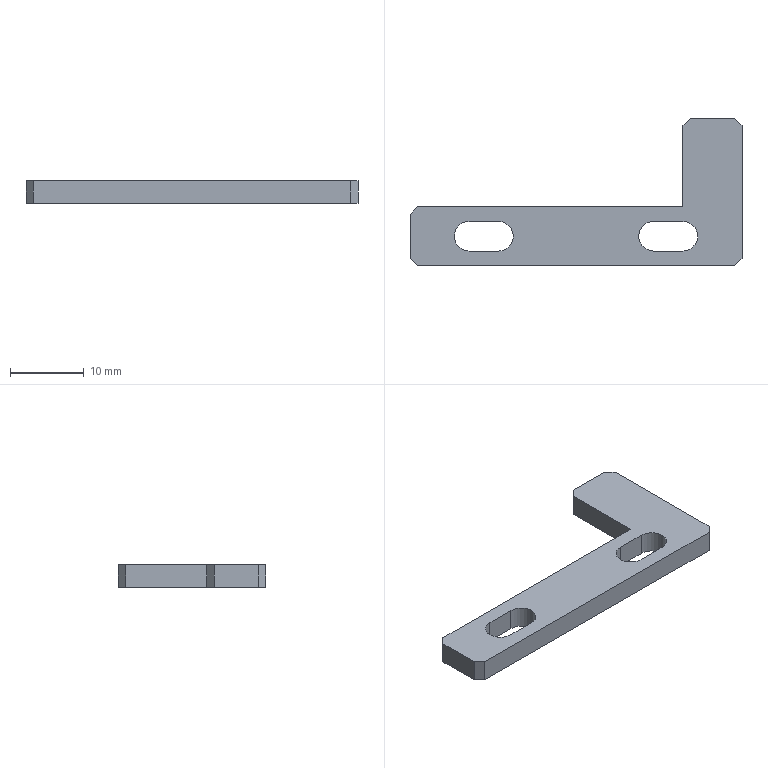Part | SolidWorks | features Chamfer 1, Extrusion 1, ICE 1 | 1 solid | 23 faces | box 45 x 20 x 3 mm | volume 1189 mm3 | plane 17 | cylinder 6 | commonest cylinder face diameters 4 x6
STEP:
#1=CARTESIAN_POINT('',(6.,4.,3.));
#2=VERTEX_POINT('',#1);
#3=CARTESIAN_POINT('',(8.,6.,3.));
#4=VERTEX_POINT('',#3);
#5=CARTESIAN_POINT('',(8.,4.,3.));
#6=DIRECTION('',(0.,0.,-1.));
#7=DIRECTION('',(-1.,0.,0.));
#8=AXIS2_PLACEMENT_3D('',#5,#6,#7);
#9=CIRCLE('',#8,2.);
#10=EDGE_CURVE('',#2,#4,#9,.T.);
#11=ORIENTED_EDGE('',*,*,#10,.F.);
#12=CARTESIAN_POINT('',(6.,4.,0.));
#13=VERTEX_POINT('',#12);
#14=CARTESIAN_POINT('',(6.,4.,3.));
#15=DIRECTION('',(0.,0.,-1.));
#16=VECTOR('',#15,1000.);
#17=LINE('',#14,#16);
#18=EDGE_CURVE('',#2,#13,#17,.T.);
#19=ORIENTED_EDGE('',*,*,#18,.T.);
#20=CARTESIAN_POINT('',(8.,6.,0.));
#21=VERTEX_POINT('',#20);
#22=CARTESIAN_POINT('',(8.,4.,0.));
#23=DIRECTION('',(0.,0.,-1.));
#24=DIRECTION('',(-1.,0.,0.));
#25=AXIS2_PLACEMENT_3D('',#22,#23,#24);
#26=CIRCLE('',#25,2.);
#27=EDGE_CURVE('',#13,#21,#26,.T.);
#28=ORIENTED_EDGE('',*,*,#27,.T.);
#29=CARTESIAN_POINT('',(8.,6.,3.));
#30=DIRECTION('',(0.,0.,-1.));
#31=VECTOR('',#30,1000.);
#32=LINE('',#29,#31);
#33=EDGE_CURVE('',#4,#21,#32,.T.);
#34=ORIENTED_EDGE('',*,*,#33,.F.);
#35=EDGE_LOOP('',(#11,#19,#28,#34));
#36=FACE_OUTER_BOUND('',#35,.T.);
#37=CARTESIAN_POINT('',(8.,4.,3.));
#38=DIRECTION('',(0.,0.,-1.));
#39=DIRECTION('',(-1.,0.,0.));
#40=AXIS2_PLACEMENT_3D('',#37,#38,#39);
#41=CYLINDRICAL_SURFACE('',#40,2.);
#42=ADVANCED_FACE('',(#36),#41,.F.);
#43=CARTESIAN_POINT('',(31.,4.,3.));
#44=VERTEX_POINT('',#43);
#45=CARTESIAN_POINT('',(33.,6.,3.));
#46=VERTEX_POINT('',#45);
#47=CARTESIAN_POINT('',(33.,4.,3.));
#48=DIRECTION('',(0.,0.,-1.));
#49=DIRECTION('',(-1.,0.,0.));
#50=AXIS2_PLACEMENT_3D('',#47,#48,#49);
#51=CIRCLE('',#50,2.);
#52=EDGE_CURVE('',#44,#46,#51,.T.);
#53=ORIENTED_EDGE('',*,*,#52,.F.);
#54=CARTESIAN_POINT('',(31.,4.,0.));
#55=VERTEX_POINT('',#54);
#56=CARTESIAN_POINT('',(31.,4.,3.));
#57=DIRECTION('',(0.,0.,-1.));
#58=VECTOR('',#57,1000.);
#59=LINE('',#56,#58);
#60=EDGE_CURVE('',#44,#55,#59,.T.);
#61=ORIENTED_EDGE('',*,*,#60,.T.);
#62=CARTESIAN_POINT('',(33.,6.,0.));
#63=VERTEX_POINT('',#62);
#64=CARTESIAN_POINT('',(33.,4.,0.));
#65=DIRECTION('',(0.,0.,-1.));
#66=DIRECTION('',(-1.,0.,0.));
#67=AXIS2_PLACEMENT_3D('',#64,#65,#66);
#68=CIRCLE('',#67,2.);
#69=EDGE_CURVE('',#55,#63,#68,.T.);
#70=ORIENTED_EDGE('',*,*,#69,.T.);
#71=CARTESIAN_POINT('',(33.,6.,3.));
#72=DIRECTION('',(0.,0.,-1.));
#73=VECTOR('',#72,1000.);
#74=LINE('',#71,#73);
#75=EDGE_CURVE('',#46,#63,#74,.T.);
#76=ORIENTED_EDGE('',*,*,#75,.F.);
#77=EDGE_LOOP('',(#53,#61,#70,#76));
#78=FACE_OUTER_BOUND('',#77,.T.);
#79=CARTESIAN_POINT('',(33.,4.,3.));
#80=DIRECTION('',(0.,0.,-1.));
#81=DIRECTION('',(-1.,0.,0.));
#82=AXIS2_PLACEMENT_3D('',#79,#80,#81);
#83=CYLINDRICAL_SURFACE('',#82,2.);
#84=ADVANCED_FACE('',(#78),#83,.F.);
#85=CARTESIAN_POINT('',(0.,7.,0.));
#86=VERTEX_POINT('',#85);
#87=CARTESIAN_POINT('',(0.,1.,0.));
#88=VERTEX_POINT('',#87);
#89=CARTESIAN_POINT('',(0.,8.,0.));
#90=DIRECTION('',(0.,-1.,0.));
#91=VECTOR('',#90,1000.);
#92=LINE('',#89,#91);
#93=EDGE_CURVE('',#86,#88,#92,.T.);
#94=ORIENTED_EDGE('',*,*,#93,.T.);
#95=CARTESIAN_POINT('',(0.,1.,3.));
#96=VERTEX_POINT('',#95);
#97=CARTESIAN_POINT('',(0.,1.,3.));
#98=DIRECTION('',(0.,0.,1.));
#99=VECTOR('',#98,1000.);
#100=LINE('',#97,#99);
#101=EDGE_CURVE('',#88,#96,#100,.T.);
#102=ORIENTED_EDGE('',*,*,#101,.T.);
#103=CARTESIAN_POINT('',(0.,7.,3.));
#104=VERTEX_POINT('',#103);
#105=CARTESIAN_POINT('',(0.,8.,3.));
#106=DIRECTION('',(0.,-1.,0.));
#107=VECTOR('',#106,1000.);
#108=LINE('',#105,#107);
#109=EDGE_CURVE('',#104,#96,#108,.T.);
#110=ORIENTED_EDGE('',*,*,#109,.F.);
#111=CARTESIAN_POINT('',(0.,7.,3.));
#112=DIRECTION('',(0.,0.,-1.));
#113=VECTOR('',#112,1000.);
#114=LINE('',#111,#113);
#115=EDGE_CURVE('',#104,#86,#114,.T.);
#116=ORIENTED_EDGE('',*,*,#115,.T.);
#117=EDGE_LOOP('',(#94,#102,#110,#116));
#118=FACE_OUTER_BOUND('',#117,.T.);
#119=CARTESIAN_POINT('',(0.,8.,3.));
#120=DIRECTION('',(1.,0.,0.));
#121=DIRECTION('',(0.,1.,0.));
#122=AXIS2_PLACEMENT_3D('',#119,#120,#121);
#123=PLANE('',#122);
#124=ADVANCED_FACE('',(#118),#123,.F.);
#125=CARTESIAN_POINT('',(1.,0.,3.));
#126=VERTEX_POINT('',#125);
#127=CARTESIAN_POINT('',(44.,0.,3.));
#128=VERTEX_POINT('',#127);
#129=CARTESIAN_POINT('',(0.,0.,3.));
#130=DIRECTION('',(1.,0.,0.));
#131=VECTOR('',#130,1000.);
#132=LINE('',#129,#131);
#133=EDGE_CURVE('',#126,#128,#132,.T.);
#134=ORIENTED_EDGE('',*,*,#133,.F.);
#135=CARTESIAN_POINT('',(1.,0.,0.));
#136=VERTEX_POINT('',#135);
#137=CARTESIAN_POINT('',(1.,0.,3.));
#138=DIRECTION('',(0.,0.,-1.));
#139=VECTOR('',#138,1000.);
#140=LINE('',#137,#139);
#141=EDGE_CURVE('',#126,#136,#140,.T.);
#142=ORIENTED_EDGE('',*,*,#141,.T.);
#143=CARTESIAN_POINT('',(44.,0.,0.));
#144=VERTEX_POINT('',#143);
#145=CARTESIAN_POINT('',(0.,0.,0.));
#146=DIRECTION('',(1.,0.,0.));
#147=VECTOR('',#146,1000.);
#148=LINE('',#145,#147);
#149=EDGE_CURVE('',#136,#144,#148,.T.);
#150=ORIENTED_EDGE('',*,*,#149,.T.);
#151=CARTESIAN_POINT('',(44.,0.,3.));
#152=DIRECTION('',(0.,0.,1.));
#153=VECTOR('',#152,1000.);
#154=LINE('',#151,#153);
#155=EDGE_CURVE('',#144,#128,#154,.T.);
#156=ORIENTED_EDGE('',*,*,#155,.T.);
#157=EDGE_LOOP('',(#134,#142,#150,#156));
#158=FACE_OUTER_BOUND('',#157,.T.);
#159=CARTESIAN_POINT('',(0.,0.,3.));
#160=DIRECTION('',(0.,1.,0.));
#161=DIRECTION('',(0.,0.,1.));
#162=AXIS2_PLACEMENT_3D('',#159,#160,#161);
#163=PLANE('',#162);
#164=ADVANCED_FACE('',(#158),#163,.F.);
#165=CARTESIAN_POINT('',(45.,1.,3.));
#166=VERTEX_POINT('',#165);
#167=CARTESIAN_POINT('',(45.,19.,3.));
#168=VERTEX_POINT('',#167);
#169=CARTESIAN_POINT('',(45.,0.,3.));
#170=DIRECTION('',(0.,1.,0.));
#171=VECTOR('',#170,1000.);
#172=LINE('',#169,#171);
#173=EDGE_CURVE('',#166,#168,#172,.T.);
#174=ORIENTED_EDGE('',*,*,#173,.F.);
#175=CARTESIAN_POINT('',(45.,1.,0.));
#176=VERTEX_POINT('',#175);
#177=CARTESIAN_POINT('',(45.,1.,3.));
#178=DIRECTION('',(0.,0.,-1.));
#179=VECTOR('',#178,1000.);
#180=LINE('',#177,#179);
#181=EDGE_CURVE('',#166,#176,#180,.T.);
#182=ORIENTED_EDGE('',*,*,#181,.T.);
#183=CARTESIAN_POINT('',(45.,19.,0.));
#184=VERTEX_POINT('',#183);
#185=CARTESIAN_POINT('',(45.,0.,0.));
#186=DIRECTION('',(0.,1.,0.));
#187=VECTOR('',#186,1000.);
#188=LINE('',#185,#187);
#189=EDGE_CURVE('',#176,#184,#188,.T.);
#190=ORIENTED_EDGE('',*,*,#189,.T.);
#191=CARTESIAN_POINT('',(45.,19.,3.));
#192=DIRECTION('',(0.,0.,1.));
#193=VECTOR('',#192,1000.);
#194=LINE('',#191,#193);
#195=EDGE_CURVE('',#184,#168,#194,.T.);
#196=ORIENTED_EDGE('',*,*,#195,.T.);
#197=EDGE_LOOP('',(#174,#182,#190,#196));
#198=FACE_OUTER_BOUND('',#197,.T.);
#199=CARTESIAN_POINT('',(45.,0.,3.));
#200=DIRECTION('',(-1.,0.,0.));
#201=DIRECTION('',(0.,0.,1.));
#202=AXIS2_PLACEMENT_3D('',#199,#200,#201);
#203=PLANE('',#202);
#204=ADVANCED_FACE('',(#198),#203,.F.);
#205=CARTESIAN_POINT('',(44.,20.,0.));
#206=VERTEX_POINT('',#205);
#207=CARTESIAN_POINT('',(38.,20.,0.));
#208=VERTEX_POINT('',#207);
#209=CARTESIAN_POINT('',(45.,20.,0.));
#210=DIRECTION('',(-1.,0.,0.));
#211=VECTOR('',#210,1000.);
#212=LINE('',#209,#211);
#213=EDGE_CURVE('',#206,#208,#212,.T.);
#214=ORIENTED_EDGE('',*,*,#213,.T.);
#215=CARTESIAN_POINT('',(38.,20.,3.));
#216=VERTEX_POINT('',#215);
#217=CARTESIAN_POINT('',(38.,20.,3.));
#218=DIRECTION('',(0.,0.,1.));
#219=VECTOR('',#218,1000.);
#220=LINE('',#217,#219);
#221=EDGE_CURVE('',#208,#216,#220,.T.);
#222=ORIENTED_EDGE('',*,*,#221,.T.);
#223=CARTESIAN_POINT('',(44.,20.,3.));
#224=VERTEX_POINT('',#223);
#225=CARTESIAN_POINT('',(45.,20.,3.));
#226=DIRECTION('',(-1.,0.,0.));
#227=VECTOR('',#226,1000.);
#228=LINE('',#225,#227);
#229=EDGE_CURVE('',#224,#216,#228,.T.);
#230=ORIENTED_EDGE('',*,*,#229,.F.);
#231=CARTESIAN_POINT('',(44.,20.,3.));
#232=DIRECTION('',(0.,0.,-1.));
#233=VECTOR('',#232,1000.);
#234=LINE('',#231,#233);
#235=EDGE_CURVE('',#224,#206,#234,.T.);
#236=ORIENTED_EDGE('',*,*,#235,.T.);
#237=EDGE_LOOP('',(#214,#222,#230,#236));
#238=FACE_OUTER_BOUND('',#237,.T.);
#239=CARTESIAN_POINT('',(45.,20.,3.));
#240=DIRECTION('',(0.,-1.,0.));
#241=DIRECTION('',(0.,0.,-1.));
#242=AXIS2_PLACEMENT_3D('',#239,#240,#241);
#243=PLANE('',#242);
#244=ADVANCED_FACE('',(#238),#243,.F.);
#245=CARTESIAN_POINT('',(37.,19.,3.));
#246=VERTEX_POINT('',#245);
#247=CARTESIAN_POINT('',(37.,8.,3.));
#248=VERTEX_POINT('',#247);
#249=CARTESIAN_POINT('',(37.,20.,3.));
#250=DIRECTION('',(0.,-1.,0.));
#251=VECTOR('',#250,1000.);
#252=LINE('',#249,#251);
#253=EDGE_CURVE('',#246,#248,#252,.T.);
#254=ORIENTED_EDGE('',*,*,#253,.F.);
#255=CARTESIAN_POINT('',(37.,19.,0.));
#256=VERTEX_POINT('',#255);
#257=CARTESIAN_POINT('',(37.,19.,3.));
#258=DIRECTION('',(0.,0.,-1.));
#259=VECTOR('',#258,1000.);
#260=LINE('',#257,#259);
#261=EDGE_CURVE('',#246,#256,#260,.T.);
#262=ORIENTED_EDGE('',*,*,#261,.T.);
#263=CARTESIAN_POINT('',(37.,8.,0.));
#264=VERTEX_POINT('',#263);
#265=CARTESIAN_POINT('',(37.,20.,0.));
#266=DIRECTION('',(0.,-1.,0.));
#267=VECTOR('',#266,1000.);
#268=LINE('',#265,#267);
#269=EDGE_CURVE('',#256,#264,#268,.T.);
#270=ORIENTED_EDGE('',*,*,#269,.T.);
#271=CARTESIAN_POINT('',(37.,8.,3.));
#272=DIRECTION('',(0.,0.,-1.));
#273=VECTOR('',#272,1000.);
#274=LINE('',#271,#273);
#275=EDGE_CURVE('',#248,#264,#274,.T.);
#276=ORIENTED_EDGE('',*,*,#275,.F.);
#277=EDGE_LOOP('',(#254,#262,#270,#276));
#278=FACE_OUTER_BOUND('',#277,.T.);
#279=CARTESIAN_POINT('',(37.,20.,3.));
#280=DIRECTION('',(1.,0.,0.));
#281=DIRECTION('',(0.,0.,-1.));
#282=AXIS2_PLACEMENT_3D('',#279,#280,#281);
#283=PLANE('',#282);
#284=ADVANCED_FACE('',(#278),#283,.F.);
#285=CARTESIAN_POINT('',(1.,8.,0.));
#286=VERTEX_POINT('',#285);
#287=CARTESIAN_POINT('',(37.,8.,0.));
#288=DIRECTION('',(-1.,0.,0.));
#289=VECTOR('',#288,1000.);
#290=LINE('',#287,#289);
#291=EDGE_CURVE('',#264,#286,#290,.T.);
#292=ORIENTED_EDGE('',*,*,#291,.T.);
#293=CARTESIAN_POINT('',(1.,8.,3.));
#294=VERTEX_POINT('',#293);
#295=CARTESIAN_POINT('',(1.,8.,3.));
#296=DIRECTION('',(0.,0.,1.));
#297=VECTOR('',#296,1000.);
#298=LINE('',#295,#297);
#299=EDGE_CURVE('',#286,#294,#298,.T.);
#300=ORIENTED_EDGE('',*,*,#299,.T.);
#301=CARTESIAN_POINT('',(37.,8.,3.));
#302=DIRECTION('',(-1.,0.,0.));
#303=VECTOR('',#302,1000.);
#304=LINE('',#301,#303);
#305=EDGE_CURVE('',#248,#294,#304,.T.);
#306=ORIENTED_EDGE('',*,*,#305,.F.);
#307=ORIENTED_EDGE('',*,*,#275,.T.);
#308=EDGE_LOOP('',(#292,#300,#306,#307));
#309=FACE_OUTER_BOUND('',#308,.T.);
#310=CARTESIAN_POINT('',(37.,8.,3.));
#311=DIRECTION('',(0.,-1.,0.));
#312=DIRECTION('',(1.,0.,0.));
#313=AXIS2_PLACEMENT_3D('',#310,#311,#312);
#314=PLANE('',#313);
#315=ADVANCED_FACE('',(#309),#314,.F.);
#316=CARTESIAN_POINT('',(12.,6.,3.));
#317=VERTEX_POINT('',#316);
#318=CARTESIAN_POINT('',(12.,2.,3.));
#319=VERTEX_POINT('',#318);
#320=CARTESIAN_POINT('',(12.,4.,3.));
#321=DIRECTION('',(0.,0.,-1.));
#322=DIRECTION('',(-1.,0.,0.));
#323=AXIS2_PLACEMENT_3D('',#320,#321,#322);
#324=CIRCLE('',#323,2.);
#325=EDGE_CURVE('',#317,#319,#324,.T.);
#326=ORIENTED_EDGE('',*,*,#325,.T.);
#327=CARTESIAN_POINT('',(8.,2.,3.));
#328=VERTEX_POINT('',#327);
#329=CARTESIAN_POINT('',(12.,2.,3.));
#330=DIRECTION('',(-1.,0.,0.));
#331=VECTOR('',#330,1000.);
#332=LINE('',#329,#331);
#333=EDGE_CURVE('',#319,#328,#332,.T.);
#334=ORIENTED_EDGE('',*,*,#333,.T.);
#335=CARTESIAN_POINT('',(8.,4.,3.));
#336=DIRECTION('',(0.,0.,-1.));
#337=DIRECTION('',(-1.,0.,0.));
#338=AXIS2_PLACEMENT_3D('',#335,#336,#337);
#339=CIRCLE('',#338,2.);
#340=EDGE_CURVE('',#328,#2,#339,.T.);
#341=ORIENTED_EDGE('',*,*,#340,.T.);
#342=ORIENTED_EDGE('',*,*,#10,.T.);
#343=CARTESIAN_POINT('',(12.,6.,3.));
#344=DIRECTION('',(1.,0.,0.));
#345=VECTOR('',#344,1000.);
#346=LINE('',#343,#345);
#347=EDGE_CURVE('',#4,#317,#346,.T.);
#348=ORIENTED_EDGE('',*,*,#347,.T.);
#349=EDGE_LOOP('',(#326,#334,#341,#342,#348));
#350=FACE_BOUND('',#349,.T.);
#351=CARTESIAN_POINT('',(37.,6.,3.));
#352=VERTEX_POINT('',#351);
#353=CARTESIAN_POINT('',(37.,2.,3.));
#354=VERTEX_POINT('',#353);
#355=CARTESIAN_POINT('',(37.,4.,3.));
#356=DIRECTION('',(0.,0.,-1.));
#357=DIRECTION('',(-1.,0.,0.));
#358=AXIS2_PLACEMENT_3D('',#355,#356,#357);
#359=CIRCLE('',#358,2.);
#360=EDGE_CURVE('',#352,#354,#359,.T.);
#361=ORIENTED_EDGE('',*,*,#360,.T.);
#362=CARTESIAN_POINT('',(33.,2.,3.));
#363=VERTEX_POINT('',#362);
#364=CARTESIAN_POINT('',(37.,2.,3.));
#365=DIRECTION('',(-1.,0.,0.));
#366=VECTOR('',#365,1000.);
#367=LINE('',#364,#366);
#368=EDGE_CURVE('',#354,#363,#367,.T.);
#369=ORIENTED_EDGE('',*,*,#368,.T.);
#370=CARTESIAN_POINT('',(33.,4.,3.));
#371=DIRECTION('',(0.,0.,-1.));
#372=DIRECTION('',(-1.,0.,0.));
#373=AXIS2_PLACEMENT_3D('',#370,#371,#372);
#374=CIRCLE('',#373,2.);
#375=EDGE_CURVE('',#363,#44,#374,.T.);
#376=ORIENTED_EDGE('',*,*,#375,.T.);
#377=ORIENTED_EDGE('',*,*,#52,.T.);
#378=CARTESIAN_POINT('',(37.,6.,3.));
#379=DIRECTION('',(1.,0.,0.));
#380=VECTOR('',#379,1000.);
#381=LINE('',#378,#380);
#382=EDGE_CURVE('',#46,#352,#381,.T.);
#383=ORIENTED_EDGE('',*,*,#382,.T.);
#384=EDGE_LOOP('',(#361,#369,#376,#377,#383));
#385=FACE_BOUND('',#384,.T.);
#386=ORIENTED_EDGE('',*,*,#109,.T.);
#387=CARTESIAN_POINT('',(0.5,0.5,3.));
#388=DIRECTION('',(0.7071,-0.7071,0.));
#389=VECTOR('',#388,1000.);
#390=LINE('',#387,#389);
#391=EDGE_CURVE('',#96,#126,#390,.T.);
#392=ORIENTED_EDGE('',*,*,#391,.T.);
#393=ORIENTED_EDGE('',*,*,#133,.T.);
#394=CARTESIAN_POINT('',(22.,-22.,3.));
#395=DIRECTION('',(0.7071,0.7071,0.));
#396=VECTOR('',#395,1000.);
#397=LINE('',#394,#396);
#398=EDGE_CURVE('',#128,#166,#397,.T.);
#399=ORIENTED_EDGE('',*,*,#398,.T.);
#400=ORIENTED_EDGE('',*,*,#173,.T.);
#401=CARTESIAN_POINT('',(32.,32.,3.));
#402=DIRECTION('',(-0.7071,0.7071,0.));
#403=VECTOR('',#402,1000.);
#404=LINE('',#401,#403);
#405=EDGE_CURVE('',#168,#224,#404,.T.);
#406=ORIENTED_EDGE('',*,*,#405,.T.);
#407=ORIENTED_EDGE('',*,*,#229,.T.);
#408=CARTESIAN_POINT('',(9.,-9.,3.));
#409=DIRECTION('',(-0.7071,-0.7071,0.));
#410=VECTOR('',#409,1000.);
#411=LINE('',#408,#410);
#412=EDGE_CURVE('',#216,#246,#411,.T.);
#413=ORIENTED_EDGE('',*,*,#412,.T.);
#414=ORIENTED_EDGE('',*,*,#253,.T.);
#415=ORIENTED_EDGE('',*,*,#305,.T.);
#416=CARTESIAN_POINT('',(-3.5,3.5,3.));
#417=DIRECTION('',(-0.7071,-0.7071,0.));
#418=VECTOR('',#417,1000.);
#419=LINE('',#416,#418);
#420=EDGE_CURVE('',#294,#104,#419,.T.);
#421=ORIENTED_EDGE('',*,*,#420,.T.);
#422=EDGE_LOOP('',(#386,#392,#393,#399,#400,#406,#407,#413,#414,#415,#421));
#423=FACE_OUTER_BOUND('',#422,.T.);
#424=CARTESIAN_POINT('',(0.,0.,3.));
#425=DIRECTION('',(0.,0.,1.));
#426=DIRECTION('',(1.,0.,0.));
#427=AXIS2_PLACEMENT_3D('',#424,#425,#426);
#428=PLANE('',#427);
#429=ADVANCED_FACE('',(#350,#385,#423),#428,.T.);
#430=CARTESIAN_POINT('',(12.,2.,0.));
#431=VERTEX_POINT('',#430);
#432=CARTESIAN_POINT('',(8.,2.,0.));
#433=VERTEX_POINT('',#432);
#434=CARTESIAN_POINT('',(12.,2.,0.));
#435=DIRECTION('',(-1.,0.,0.));
#436=VECTOR('',#435,1000.);
#437=LINE('',#434,#436);
#438=EDGE_CURVE('',#431,#433,#437,.T.);
#439=ORIENTED_EDGE('',*,*,#438,.F.);
#440=CARTESIAN_POINT('',(12.,6.,0.));
#441=VERTEX_POINT('',#440);
#442=CARTESIAN_POINT('',(12.,4.,0.));
#443=DIRECTION('',(0.,0.,-1.));
#444=DIRECTION('',(-1.,0.,0.));
#445=AXIS2_PLACEMENT_3D('',#442,#443,#444);
#446=CIRCLE('',#445,2.);
#447=EDGE_CURVE('',#441,#431,#446,.T.);
#448=ORIENTED_EDGE('',*,*,#447,.F.);
#449=CARTESIAN_POINT('',(12.,6.,0.));
#450=DIRECTION('',(1.,0.,0.));
#451=VECTOR('',#450,1000.);
#452=LINE('',#449,#451);
#453=EDGE_CURVE('',#21,#441,#452,.T.);
#454=ORIENTED_EDGE('',*,*,#453,.F.);
#455=ORIENTED_EDGE('',*,*,#27,.F.);
#456=CARTESIAN_POINT('',(8.,4.,0.));
#457=DIRECTION('',(0.,0.,-1.));
#458=DIRECTION('',(-1.,0.,0.));
#459=AXIS2_PLACEMENT_3D('',#456,#457,#458);
#460=CIRCLE('',#459,2.);
#461=EDGE_CURVE('',#433,#13,#460,.T.);
#462=ORIENTED_EDGE('',*,*,#461,.F.);
#463=EDGE_LOOP('',(#439,#448,#454,#455,#462));
#464=FACE_BOUND('',#463,.T.);
#465=CARTESIAN_POINT('',(37.,2.,0.));
#466=VERTEX_POINT('',#465);
#467=CARTESIAN_POINT('',(33.,2.,0.));
#468=VERTEX_POINT('',#467);
#469=CARTESIAN_POINT('',(37.,2.,0.));
#470=DIRECTION('',(-1.,0.,0.));
#471=VECTOR('',#470,1000.);
#472=LINE('',#469,#471);
#473=EDGE_CURVE('',#466,#468,#472,.T.);
#474=ORIENTED_EDGE('',*,*,#473,.F.);
#475=CARTESIAN_POINT('',(37.,6.,0.));
#476=VERTEX_POINT('',#475);
#477=CARTESIAN_POINT('',(37.,4.,0.));
#478=DIRECTION('',(0.,0.,-1.));
#479=DIRECTION('',(-1.,0.,0.));
#480=AXIS2_PLACEMENT_3D('',#477,#478,#479);
#481=CIRCLE('',#480,2.);
#482=EDGE_CURVE('',#476,#466,#481,.T.);
#483=ORIENTED_EDGE('',*,*,#482,.F.);
#484=CARTESIAN_POINT('',(37.,6.,0.));
#485=DIRECTION('',(1.,0.,0.));
#486=VECTOR('',#485,1000.);
#487=LINE('',#484,#486);
#488=EDGE_CURVE('',#63,#476,#487,.T.);
#489=ORIENTED_EDGE('',*,*,#488,.F.);
#490=ORIENTED_EDGE('',*,*,#69,.F.);
#491=CARTESIAN_POINT('',(33.,4.,0.));
#492=DIRECTION('',(0.,0.,-1.));
#493=DIRECTION('',(-1.,0.,0.));
#494=AXIS2_PLACEMENT_3D('',#491,#492,#493);
#495=CIRCLE('',#494,2.);
#496=EDGE_CURVE('',#468,#55,#495,.T.);
#497=ORIENTED_EDGE('',*,*,#496,.F.);
#498=EDGE_LOOP('',(#474,#483,#489,#490,#497));
#499=FACE_BOUND('',#498,.T.);
#500=ORIENTED_EDGE('',*,*,#149,.F.);
#501=CARTESIAN_POINT('',(1.,0.,0.));
#502=DIRECTION('',(-0.7071,0.7071,0.));
#503=VECTOR('',#502,1000.);
#504=LINE('',#501,#503);
#505=EDGE_CURVE('',#136,#88,#504,.T.);
#506=ORIENTED_EDGE('',*,*,#505,.T.);
#507=ORIENTED_EDGE('',*,*,#93,.F.);
#508=CARTESIAN_POINT('',(0.,7.,0.));
#509=DIRECTION('',(0.7071,0.7071,0.));
#510=VECTOR('',#509,1000.);
#511=LINE('',#508,#510);
#512=EDGE_CURVE('',#86,#286,#511,.T.);
#513=ORIENTED_EDGE('',*,*,#512,.T.);
#514=ORIENTED_EDGE('',*,*,#291,.F.);
#515=ORIENTED_EDGE('',*,*,#269,.F.);
#516=CARTESIAN_POINT('',(37.,19.,0.));
#517=DIRECTION('',(0.7071,0.7071,0.));
#518=VECTOR('',#517,1000.);
#519=LINE('',#516,#518);
#520=EDGE_CURVE('',#256,#208,#519,.T.);
#521=ORIENTED_EDGE('',*,*,#520,.T.);
#522=ORIENTED_EDGE('',*,*,#213,.F.);
#523=CARTESIAN_POINT('',(44.,20.,0.));
#524=DIRECTION('',(0.7071,-0.7071,0.));
#525=VECTOR('',#524,1000.);
#526=LINE('',#523,#525);
#527=EDGE_CURVE('',#206,#184,#526,.T.);
#528=ORIENTED_EDGE('',*,*,#527,.T.);
#529=ORIENTED_EDGE('',*,*,#189,.F.);
#530=CARTESIAN_POINT('',(45.,1.,0.));
#531=DIRECTION('',(-0.7071,-0.7071,0.));
#532=VECTOR('',#531,1000.);
#533=LINE('',#530,#532);
#534=EDGE_CURVE('',#176,#144,#533,.T.);
#535=ORIENTED_EDGE('',*,*,#534,.T.);
#536=EDGE_LOOP('',(#500,#506,#507,#513,#514,#515,#521,#522,#528,#529,#535));
#537=FACE_OUTER_BOUND('',#536,.T.);
#538=CARTESIAN_POINT('',(0.,0.,0.));
#539=DIRECTION('',(0.,0.,1.));
#540=DIRECTION('',(1.,0.,0.));
#541=AXIS2_PLACEMENT_3D('',#538,#539,#540);
#542=PLANE('',#541);
#543=ADVANCED_FACE('',(#464,#499,#537),#542,.F.);
#544=ORIENTED_EDGE('',*,*,#482,.T.);
#545=CARTESIAN_POINT('',(37.,2.,3.));
#546=DIRECTION('',(0.,0.,-1.));
#547=VECTOR('',#546,1000.);
#548=LINE('',#545,#547);
#549=EDGE_CURVE('',#354,#466,#548,.T.);
#550=ORIENTED_EDGE('',*,*,#549,.F.);
#551=ORIENTED_EDGE('',*,*,#360,.F.);
#552=CARTESIAN_POINT('',(37.,6.,3.));
#553=DIRECTION('',(0.,0.,-1.));
#554=VECTOR('',#553,1000.);
#555=LINE('',#552,#554);
#556=EDGE_CURVE('',#352,#476,#555,.T.);
#557=ORIENTED_EDGE('',*,*,#556,.T.);
#558=EDGE_LOOP('',(#544,#550,#551,#557));
#559=FACE_OUTER_BOUND('',#558,.T.);
#560=CARTESIAN_POINT('',(37.,4.,3.));
#561=DIRECTION('',(0.,0.,-1.));
#562=DIRECTION('',(-1.,0.,0.));
#563=AXIS2_PLACEMENT_3D('',#560,#561,#562);
#564=CYLINDRICAL_SURFACE('',#563,2.);
#565=ADVANCED_FACE('',(#559),#564,.F.);
#566=ORIENTED_EDGE('',*,*,#488,.T.);
#567=ORIENTED_EDGE('',*,*,#556,.F.);
#568=ORIENTED_EDGE('',*,*,#382,.F.);
#569=ORIENTED_EDGE('',*,*,#75,.T.);
#570=EDGE_LOOP('',(#566,#567,#568,#569));
#571=FACE_OUTER_BOUND('',#570,.T.);
#572=CARTESIAN_POINT('',(37.,6.,3.));
#573=DIRECTION('',(0.,1.,0.));
#574=DIRECTION('',(-1.,0.,0.));
#575=AXIS2_PLACEMENT_3D('',#572,#573,#574);
#576=PLANE('',#575);
#577=ADVANCED_FACE('',(#571),#576,.F.);
#578=ORIENTED_EDGE('',*,*,#60,.F.);
#579=ORIENTED_EDGE('',*,*,#375,.F.);
#580=CARTESIAN_POINT('',(33.,2.,3.));
#581=DIRECTION('',(0.,0.,-1.));
#582=VECTOR('',#581,1000.);
#583=LINE('',#580,#582);
#584=EDGE_CURVE('',#363,#468,#583,.T.);
#585=ORIENTED_EDGE('',*,*,#584,.T.);
#586=ORIENTED_EDGE('',*,*,#496,.T.);
#587=EDGE_LOOP('',(#578,#579,#585,#586));
#588=FACE_OUTER_BOUND('',#587,.T.);
#589=CARTESIAN_POINT('',(33.,4.,3.));
#590=DIRECTION('',(0.,0.,-1.));
#591=DIRECTION('',(-1.,0.,0.));
#592=AXIS2_PLACEMENT_3D('',#589,#590,#591);
#593=CYLINDRICAL_SURFACE('',#592,2.);
#594=ADVANCED_FACE('',(#588),#593,.F.);
#595=ORIENTED_EDGE('',*,*,#473,.T.);
#596=ORIENTED_EDGE('',*,*,#584,.F.);
#597=ORIENTED_EDGE('',*,*,#368,.F.);
#598=ORIENTED_EDGE('',*,*,#549,.T.);
#599=EDGE_LOOP('',(#595,#596,#597,#598));
#600=FACE_OUTER_BOUND('',#599,.T.);
#601=CARTESIAN_POINT('',(37.,2.,3.));
#602=DIRECTION('',(0.,-1.,0.));
#603=DIRECTION('',(1.,0.,0.));
#604=AXIS2_PLACEMENT_3D('',#601,#602,#603);
#605=PLANE('',#604);
#606=ADVANCED_FACE('',(#600),#605,.F.);
#607=ORIENTED_EDGE('',*,*,#447,.T.);
#608=CARTESIAN_POINT('',(12.,2.,3.));
#609=DIRECTION('',(0.,0.,-1.));
#610=VECTOR('',#609,1000.);
#611=LINE('',#608,#610);
#612=EDGE_CURVE('',#319,#431,#611,.T.);
#613=ORIENTED_EDGE('',*,*,#612,.F.);
#614=ORIENTED_EDGE('',*,*,#325,.F.);
#615=CARTESIAN_POINT('',(12.,6.,3.));
#616=DIRECTION('',(0.,0.,-1.));
#617=VECTOR('',#616,1000.);
#618=LINE('',#615,#617);
#619=EDGE_CURVE('',#317,#441,#618,.T.);
#620=ORIENTED_EDGE('',*,*,#619,.T.);
#621=EDGE_LOOP('',(#607,#613,#614,#620));
#622=FACE_OUTER_BOUND('',#621,.T.);
#623=CARTESIAN_POINT('',(12.,4.,3.));
#624=DIRECTION('',(0.,0.,-1.));
#625=DIRECTION('',(-1.,0.,0.));
#626=AXIS2_PLACEMENT_3D('',#623,#624,#625);
#627=CYLINDRICAL_SURFACE('',#626,2.);
#628=ADVANCED_FACE('',(#622),#627,.F.);
#629=ORIENTED_EDGE('',*,*,#453,.T.);
#630=ORIENTED_EDGE('',*,*,#619,.F.);
#631=ORIENTED_EDGE('',*,*,#347,.F.);
#632=ORIENTED_EDGE('',*,*,#33,.T.);
#633=EDGE_LOOP('',(#629,#630,#631,#632));
#634=FACE_OUTER_BOUND('',#633,.T.);
#635=CARTESIAN_POINT('',(12.,6.,3.));
#636=DIRECTION('',(0.,1.,0.));
#637=DIRECTION('',(-1.,0.,0.));
#638=AXIS2_PLACEMENT_3D('',#635,#636,#637);
#639=PLANE('',#638);
#640=ADVANCED_FACE('',(#634),#639,.F.);
#641=ORIENTED_EDGE('',*,*,#18,.F.);
#642=ORIENTED_EDGE('',*,*,#340,.F.);
#643=CARTESIAN_POINT('',(8.,2.,3.));
#644=DIRECTION('',(0.,0.,-1.));
#645=VECTOR('',#644,1000.);
#646=LINE('',#643,#645);
#647=EDGE_CURVE('',#328,#433,#646,.T.);
#648=ORIENTED_EDGE('',*,*,#647,.T.);
#649=ORIENTED_EDGE('',*,*,#461,.T.);
#650=EDGE_LOOP('',(#641,#642,#648,#649));
#651=FACE_OUTER_BOUND('',#650,.T.);
#652=CARTESIAN_POINT('',(8.,4.,3.));
#653=DIRECTION('',(0.,0.,-1.));
#654=DIRECTION('',(-1.,0.,0.));
#655=AXIS2_PLACEMENT_3D('',#652,#653,#654);
#656=CYLINDRICAL_SURFACE('',#655,2.);
#657=ADVANCED_FACE('',(#651),#656,.F.);
#658=ORIENTED_EDGE('',*,*,#438,.T.);
#659=ORIENTED_EDGE('',*,*,#647,.F.);
#660=ORIENTED_EDGE('',*,*,#333,.F.);
#661=ORIENTED_EDGE('',*,*,#612,.T.);
#662=EDGE_LOOP('',(#658,#659,#660,#661));
#663=FACE_OUTER_BOUND('',#662,.T.);
#664=CARTESIAN_POINT('',(12.,2.,3.));
#665=DIRECTION('',(0.,-1.,0.));
#666=DIRECTION('',(1.,0.,0.));
#667=AXIS2_PLACEMENT_3D('',#664,#665,#666);
#668=PLANE('',#667);
#669=ADVANCED_FACE('',(#663),#668,.F.);
#670=ORIENTED_EDGE('',*,*,#391,.F.);
#671=ORIENTED_EDGE('',*,*,#101,.F.);
#672=ORIENTED_EDGE('',*,*,#505,.F.);
#673=ORIENTED_EDGE('',*,*,#141,.F.);
#674=EDGE_LOOP('',(#670,#671,#672,#673));
#675=FACE_OUTER_BOUND('',#674,.T.);
#676=CARTESIAN_POINT('',(1.,0.,3.));
#677=DIRECTION('',(0.7071,0.7071,0.));
#678=DIRECTION('',(0.,0.,-1.));
#679=AXIS2_PLACEMENT_3D('',#676,#677,#678);
#680=PLANE('',#679);
#681=ADVANCED_FACE('',(#675),#680,.F.);
#682=ORIENTED_EDGE('',*,*,#420,.F.);
#683=ORIENTED_EDGE('',*,*,#299,.F.);
#684=ORIENTED_EDGE('',*,*,#512,.F.);
#685=ORIENTED_EDGE('',*,*,#115,.F.);
#686=EDGE_LOOP('',(#682,#683,#684,#685));
#687=FACE_OUTER_BOUND('',#686,.T.);
#688=CARTESIAN_POINT('',(0.,7.,3.));
#689=DIRECTION('',(0.7071,-0.7071,0.));
#690=DIRECTION('',(0.,0.,-1.));
#691=AXIS2_PLACEMENT_3D('',#688,#689,#690);
#692=PLANE('',#691);
#693=ADVANCED_FACE('',(#687),#692,.F.);
#694=ORIENTED_EDGE('',*,*,#412,.F.);
#695=ORIENTED_EDGE('',*,*,#221,.F.);
#696=ORIENTED_EDGE('',*,*,#520,.F.);
#697=ORIENTED_EDGE('',*,*,#261,.F.);
#698=EDGE_LOOP('',(#694,#695,#696,#697));
#699=FACE_OUTER_BOUND('',#698,.T.);
#700=CARTESIAN_POINT('',(37.,19.,3.));
#701=DIRECTION('',(0.7071,-0.7071,0.));
#702=DIRECTION('',(0.,0.,-1.));
#703=AXIS2_PLACEMENT_3D('',#700,#701,#702);
#704=PLANE('',#703);
#705=ADVANCED_FACE('',(#699),#704,.F.);
#706=ORIENTED_EDGE('',*,*,#398,.F.);
#707=ORIENTED_EDGE('',*,*,#155,.F.);
#708=ORIENTED_EDGE('',*,*,#534,.F.);
#709=ORIENTED_EDGE('',*,*,#181,.F.);
#710=EDGE_LOOP('',(#706,#707,#708,#709));
#711=FACE_OUTER_BOUND('',#710,.T.);
#712=CARTESIAN_POINT('',(45.,1.,3.));
#713=DIRECTION('',(-0.7071,0.7071,0.));
#714=DIRECTION('',(0.,0.,-1.));
#715=AXIS2_PLACEMENT_3D('',#712,#713,#714);
#716=PLANE('',#715);
#717=ADVANCED_FACE('',(#711),#716,.F.);
#718=ORIENTED_EDGE('',*,*,#405,.F.);
#719=ORIENTED_EDGE('',*,*,#195,.F.);
#720=ORIENTED_EDGE('',*,*,#527,.F.);
#721=ORIENTED_EDGE('',*,*,#235,.F.);
#722=EDGE_LOOP('',(#718,#719,#720,#721));
#723=FACE_OUTER_BOUND('',#722,.T.);
#724=CARTESIAN_POINT('',(44.,20.,3.));
#725=DIRECTION('',(-0.7071,-0.7071,0.));
#726=DIRECTION('',(0.,0.,-1.));
#727=AXIS2_PLACEMENT_3D('',#724,#725,#726);
#728=PLANE('',#727);
#729=ADVANCED_FACE('',(#723),#728,.F.);
#730=CLOSED_SHELL('',(#42,#84,#124,#164,#204,#244,#284,#315,#429,#543,#565,#577,#594,#606,#628,#640,#657,#669,#681,#693,#705,#717,#729));
#731=MANIFOLD_SOLID_BREP('',#730);
#732=CARTESIAN_POINT('',(0.,0.,0.));
#733=DIRECTION('',(0.,0.,1.));
#734=DIRECTION('',(1.,0.,0.));
#735=AXIS2_PLACEMENT_3D('',#732,#733,#734);
#736=(LENGTH_UNIT()NAMED_UNIT(*)SI_UNIT(.MILLI.,.METRE.));
#737=UNCERTAINTY_MEASURE_WITH_UNIT(LENGTH_MEASURE(0.00001),#736,'','');
#738=(NAMED_UNIT(*)PLANE_ANGLE_UNIT()SI_UNIT($,.RADIAN.));
#739=(NAMED_UNIT(*)SI_UNIT($,.STERADIAN.)SOLID_ANGLE_UNIT());
#740=(GEOMETRIC_REPRESENTATION_CONTEXT(3)GLOBAL_UNCERTAINTY_ASSIGNED_CONTEXT((#737))GLOBAL_UNIT_ASSIGNED_CONTEXT((#736,#738,#739))REPRESENTATION_CONTEXT('',''));
#741=ADVANCED_BREP_SHAPE_REPRESENTATION('',(#731,#735),#740);